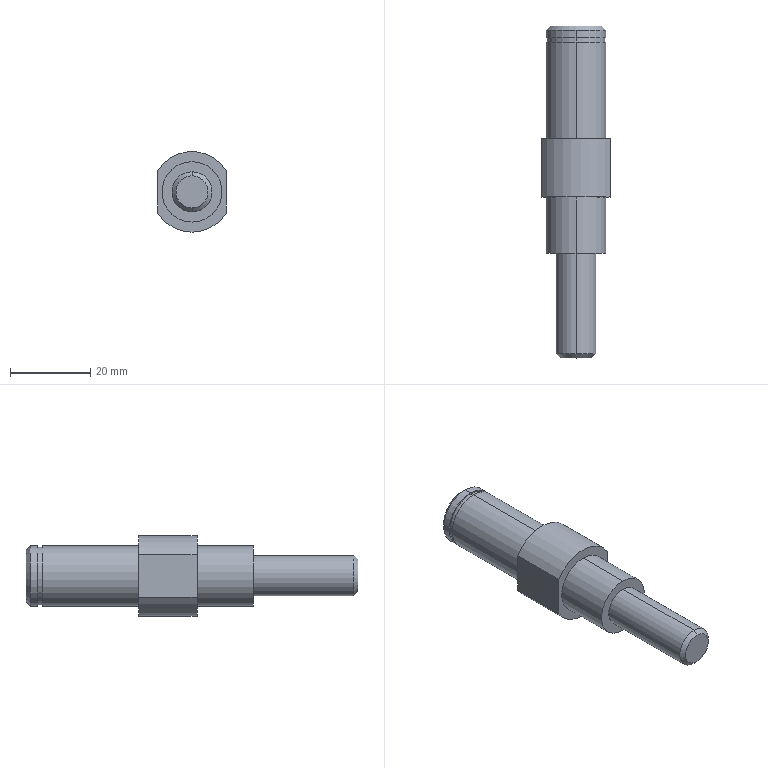Part | STEP file | Driven wheel shaft | 1 solid | 26 faces | box 17 x 82.5 x 20 mm | volume 13654 mm3 | cylinder 13 | plane 9 | cone 4 | commonest cylinder face diameters 15 x6 20 x3 10 x2 14.3 x2